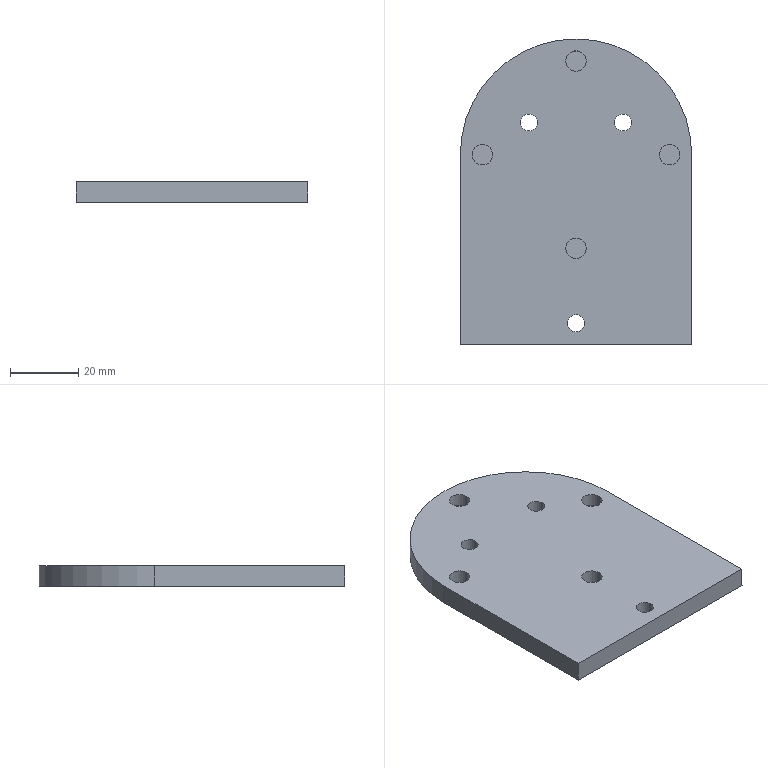Part | SolidWorks | features Cut 2, Extrusion 1 | 1 solid | 24 faces | box 68 x 89.927 x 6 mm | volume 32907 mm3 | cylinder 15 | plane 9 | commonest cylinder face diameters 6 x8 5 x6 68 x1
STEP:
#1=CARTESIAN_POINT('',(-43.159,19.21,6.));
#2=VERTEX_POINT('',#1);
#3=CARTESIAN_POINT('',(-48.159,19.21,6.));
#4=VERTEX_POINT('',#3);
#5=CARTESIAN_POINT('',(-45.659,19.21,6.));
#6=DIRECTION('',(0.,0.,-1.));
#7=DIRECTION('',(-1.,0.,0.));
#8=AXIS2_PLACEMENT_3D('',#5,#6,#7);
#9=CIRCLE('',#8,2.5);
#10=EDGE_CURVE('',#2,#4,#9,.T.);
#11=ORIENTED_EDGE('',*,*,#10,.F.);
#12=CARTESIAN_POINT('',(-43.159,19.21,0.));
#13=VERTEX_POINT('',#12);
#14=CARTESIAN_POINT('',(-43.159,19.21,6.));
#15=DIRECTION('',(0.,0.,-1.));
#16=VECTOR('',#15,1000.);
#17=LINE('',#14,#16);
#18=EDGE_CURVE('',#2,#13,#17,.T.);
#19=ORIENTED_EDGE('',*,*,#18,.T.);
#20=CARTESIAN_POINT('',(-48.159,19.21,0.));
#21=VERTEX_POINT('',#20);
#22=CARTESIAN_POINT('',(-45.659,19.21,0.));
#23=DIRECTION('',(0.,0.,-1.));
#24=DIRECTION('',(-1.,0.,0.));
#25=AXIS2_PLACEMENT_3D('',#22,#23,#24);
#26=CIRCLE('',#25,2.5);
#27=EDGE_CURVE('',#13,#21,#26,.T.);
#28=ORIENTED_EDGE('',*,*,#27,.T.);
#29=CARTESIAN_POINT('',(-48.159,19.21,6.));
#30=DIRECTION('',(0.,0.,-1.));
#31=VECTOR('',#30,1000.);
#32=LINE('',#29,#31);
#33=EDGE_CURVE('',#4,#21,#32,.T.);
#34=ORIENTED_EDGE('',*,*,#33,.F.);
#35=EDGE_LOOP('',(#11,#19,#28,#34));
#36=FACE_OUTER_BOUND('',#35,.T.);
#37=CARTESIAN_POINT('',(-45.659,19.21,6.));
#38=DIRECTION('',(0.,0.,-1.));
#39=DIRECTION('',(-1.,0.,0.));
#40=AXIS2_PLACEMENT_3D('',#37,#38,#39);
#41=CYLINDRICAL_SURFACE('',#40,2.5);
#42=ADVANCED_FACE('',(#36),#41,.F.);
#43=CARTESIAN_POINT('',(-15.478,19.21,6.));
#44=VERTEX_POINT('',#43);
#45=CARTESIAN_POINT('',(-20.478,19.21,6.));
#46=VERTEX_POINT('',#45);
#47=CARTESIAN_POINT('',(-17.978,19.21,6.));
#48=DIRECTION('',(0.,0.,-1.));
#49=DIRECTION('',(-1.,0.,0.));
#50=AXIS2_PLACEMENT_3D('',#47,#48,#49);
#51=CIRCLE('',#50,2.5);
#52=EDGE_CURVE('',#44,#46,#51,.T.);
#53=ORIENTED_EDGE('',*,*,#52,.F.);
#54=CARTESIAN_POINT('',(-15.478,19.21,0.));
#55=VERTEX_POINT('',#54);
#56=CARTESIAN_POINT('',(-15.478,19.21,6.));
#57=DIRECTION('',(0.,0.,-1.));
#58=VECTOR('',#57,1000.);
#59=LINE('',#56,#58);
#60=EDGE_CURVE('',#44,#55,#59,.T.);
#61=ORIENTED_EDGE('',*,*,#60,.T.);
#62=CARTESIAN_POINT('',(-20.478,19.21,0.));
#63=VERTEX_POINT('',#62);
#64=CARTESIAN_POINT('',(-17.978,19.21,0.));
#65=DIRECTION('',(0.,0.,-1.));
#66=DIRECTION('',(-1.,0.,0.));
#67=AXIS2_PLACEMENT_3D('',#64,#65,#66);
#68=CIRCLE('',#67,2.5);
#69=EDGE_CURVE('',#55,#63,#68,.T.);
#70=ORIENTED_EDGE('',*,*,#69,.T.);
#71=CARTESIAN_POINT('',(-20.478,19.21,6.));
#72=DIRECTION('',(0.,0.,-1.));
#73=VECTOR('',#72,1000.);
#74=LINE('',#71,#73);
#75=EDGE_CURVE('',#46,#63,#74,.T.);
#76=ORIENTED_EDGE('',*,*,#75,.F.);
#77=EDGE_LOOP('',(#53,#61,#70,#76));
#78=FACE_OUTER_BOUND('',#77,.T.);
#79=CARTESIAN_POINT('',(-17.978,19.21,6.));
#80=DIRECTION('',(0.,0.,-1.));
#81=DIRECTION('',(-1.,0.,0.));
#82=AXIS2_PLACEMENT_3D('',#79,#80,#81);
#83=CYLINDRICAL_SURFACE('',#82,2.5);
#84=ADVANCED_FACE('',(#78),#83,.F.);
#85=CARTESIAN_POINT('',(-29.318,-39.754,6.));
#86=VERTEX_POINT('',#85);
#87=CARTESIAN_POINT('',(-34.318,-39.754,6.));
#88=VERTEX_POINT('',#87);
#89=CARTESIAN_POINT('',(-31.818,-39.754,6.));
#90=DIRECTION('',(0.,0.,-1.));
#91=DIRECTION('',(-1.,0.,0.));
#92=AXIS2_PLACEMENT_3D('',#89,#90,#91);
#93=CIRCLE('',#92,2.5);
#94=EDGE_CURVE('',#86,#88,#93,.T.);
#95=ORIENTED_EDGE('',*,*,#94,.F.);
#96=CARTESIAN_POINT('',(-29.318,-39.754,0.));
#97=VERTEX_POINT('',#96);
#98=CARTESIAN_POINT('',(-29.318,-39.754,6.));
#99=DIRECTION('',(0.,0.,-1.));
#100=VECTOR('',#99,1000.);
#101=LINE('',#98,#100);
#102=EDGE_CURVE('',#86,#97,#101,.T.);
#103=ORIENTED_EDGE('',*,*,#102,.T.);
#104=CARTESIAN_POINT('',(-34.318,-39.754,0.));
#105=VERTEX_POINT('',#104);
#106=CARTESIAN_POINT('',(-31.818,-39.754,0.));
#107=DIRECTION('',(0.,0.,-1.));
#108=DIRECTION('',(-1.,0.,0.));
#109=AXIS2_PLACEMENT_3D('',#106,#107,#108);
#110=CIRCLE('',#109,2.5);
#111=EDGE_CURVE('',#97,#105,#110,.T.);
#112=ORIENTED_EDGE('',*,*,#111,.T.);
#113=CARTESIAN_POINT('',(-34.318,-39.754,6.));
#114=DIRECTION('',(0.,0.,-1.));
#115=VECTOR('',#114,1000.);
#116=LINE('',#113,#115);
#117=EDGE_CURVE('',#88,#105,#116,.T.);
#118=ORIENTED_EDGE('',*,*,#117,.F.);
#119=EDGE_LOOP('',(#95,#103,#112,#118));
#120=FACE_OUTER_BOUND('',#119,.T.);
#121=CARTESIAN_POINT('',(-31.818,-39.754,6.));
#122=DIRECTION('',(0.,0.,-1.));
#123=DIRECTION('',(-1.,0.,0.));
#124=AXIS2_PLACEMENT_3D('',#121,#122,#123);
#125=CYLINDRICAL_SURFACE('',#124,2.5);
#126=ADVANCED_FACE('',(#120),#125,.F.);
#127=CARTESIAN_POINT('',(-34.818,37.244,2.));
#128=VERTEX_POINT('',#127);
#129=CARTESIAN_POINT('',(-28.818,37.244,2.));
#130=VERTEX_POINT('',#129);
#131=CARTESIAN_POINT('',(-31.818,37.244,2.));
#132=DIRECTION('',(0.,0.,1.));
#133=DIRECTION('',(1.,0.,0.));
#134=AXIS2_PLACEMENT_3D('',#131,#132,#133);
#135=CIRCLE('',#134,3.);
#136=EDGE_CURVE('',#128,#130,#135,.T.);
#137=ORIENTED_EDGE('',*,*,#136,.F.);
#138=CARTESIAN_POINT('',(-34.818,37.244,6.));
#139=VERTEX_POINT('',#138);
#140=CARTESIAN_POINT('',(-34.818,37.244,2.));
#141=DIRECTION('',(0.,0.,1.));
#142=VECTOR('',#141,1000.);
#143=LINE('',#140,#142);
#144=EDGE_CURVE('',#128,#139,#143,.T.);
#145=ORIENTED_EDGE('',*,*,#144,.T.);
#146=CARTESIAN_POINT('',(-28.818,37.244,6.));
#147=VERTEX_POINT('',#146);
#148=CARTESIAN_POINT('',(-31.818,37.244,6.));
#149=DIRECTION('',(0.,0.,1.));
#150=DIRECTION('',(1.,0.,0.));
#151=AXIS2_PLACEMENT_3D('',#148,#149,#150);
#152=CIRCLE('',#151,3.);
#153=EDGE_CURVE('',#139,#147,#152,.T.);
#154=ORIENTED_EDGE('',*,*,#153,.T.);
#155=CARTESIAN_POINT('',(-28.818,37.244,2.));
#156=DIRECTION('',(0.,0.,1.));
#157=VECTOR('',#156,1000.);
#158=LINE('',#155,#157);
#159=EDGE_CURVE('',#130,#147,#158,.T.);
#160=ORIENTED_EDGE('',*,*,#159,.F.);
#161=EDGE_LOOP('',(#137,#145,#154,#160));
#162=FACE_OUTER_BOUND('',#161,.T.);
#163=CARTESIAN_POINT('',(-31.818,37.244,2.));
#164=DIRECTION('',(0.,0.,1.));
#165=DIRECTION('',(1.,0.,0.));
#166=AXIS2_PLACEMENT_3D('',#163,#164,#165);
#167=CYLINDRICAL_SURFACE('',#166,3.);
#168=ADVANCED_FACE('',(#162),#167,.F.);
#169=CARTESIAN_POINT('',(-7.318,9.744,2.));
#170=VERTEX_POINT('',#169);
#171=CARTESIAN_POINT('',(-1.318,9.744,2.));
#172=VERTEX_POINT('',#171);
#173=CARTESIAN_POINT('',(-4.318,9.744,2.));
#174=DIRECTION('',(0.,0.,1.));
#175=DIRECTION('',(1.,0.,0.));
#176=AXIS2_PLACEMENT_3D('',#173,#174,#175);
#177=CIRCLE('',#176,3.);
#178=EDGE_CURVE('',#170,#172,#177,.T.);
#179=ORIENTED_EDGE('',*,*,#178,.F.);
#180=CARTESIAN_POINT('',(-7.318,9.744,6.));
#181=VERTEX_POINT('',#180);
#182=CARTESIAN_POINT('',(-7.318,9.744,2.));
#183=DIRECTION('',(0.,0.,1.));
#184=VECTOR('',#183,1000.);
#185=LINE('',#182,#184);
#186=EDGE_CURVE('',#170,#181,#185,.T.);
#187=ORIENTED_EDGE('',*,*,#186,.T.);
#188=CARTESIAN_POINT('',(-1.318,9.744,6.));
#189=VERTEX_POINT('',#188);
#190=CARTESIAN_POINT('',(-4.318,9.744,6.));
#191=DIRECTION('',(0.,0.,1.));
#192=DIRECTION('',(1.,0.,0.));
#193=AXIS2_PLACEMENT_3D('',#190,#191,#192);
#194=CIRCLE('',#193,3.);
#195=EDGE_CURVE('',#181,#189,#194,.T.);
#196=ORIENTED_EDGE('',*,*,#195,.T.);
#197=CARTESIAN_POINT('',(-1.318,9.744,2.));
#198=DIRECTION('',(0.,0.,1.));
#199=VECTOR('',#198,1000.);
#200=LINE('',#197,#199);
#201=EDGE_CURVE('',#172,#189,#200,.T.);
#202=ORIENTED_EDGE('',*,*,#201,.F.);
#203=EDGE_LOOP('',(#179,#187,#196,#202));
#204=FACE_OUTER_BOUND('',#203,.T.);
#205=CARTESIAN_POINT('',(-4.318,9.744,2.));
#206=DIRECTION('',(0.,0.,1.));
#207=DIRECTION('',(1.,0.,0.));
#208=AXIS2_PLACEMENT_3D('',#205,#206,#207);
#209=CYLINDRICAL_SURFACE('',#208,3.);
#210=ADVANCED_FACE('',(#204),#209,.F.);
#211=CARTESIAN_POINT('',(-34.818,-17.756,2.));
#212=VERTEX_POINT('',#211);
#213=CARTESIAN_POINT('',(-28.818,-17.756,2.));
#214=VERTEX_POINT('',#213);
#215=CARTESIAN_POINT('',(-31.818,-17.756,2.));
#216=DIRECTION('',(0.,0.,1.));
#217=DIRECTION('',(1.,0.,0.));
#218=AXIS2_PLACEMENT_3D('',#215,#216,#217);
#219=CIRCLE('',#218,3.);
#220=EDGE_CURVE('',#212,#214,#219,.T.);
#221=ORIENTED_EDGE('',*,*,#220,.F.);
#222=CARTESIAN_POINT('',(-34.818,-17.756,6.));
#223=VERTEX_POINT('',#222);
#224=CARTESIAN_POINT('',(-34.818,-17.756,2.));
#225=DIRECTION('',(0.,0.,1.));
#226=VECTOR('',#225,1000.);
#227=LINE('',#224,#226);
#228=EDGE_CURVE('',#212,#223,#227,.T.);
#229=ORIENTED_EDGE('',*,*,#228,.T.);
#230=CARTESIAN_POINT('',(-28.818,-17.756,6.));
#231=VERTEX_POINT('',#230);
#232=CARTESIAN_POINT('',(-31.818,-17.756,6.));
#233=DIRECTION('',(0.,0.,1.));
#234=DIRECTION('',(1.,0.,0.));
#235=AXIS2_PLACEMENT_3D('',#232,#233,#234);
#236=CIRCLE('',#235,3.);
#237=EDGE_CURVE('',#223,#231,#236,.T.);
#238=ORIENTED_EDGE('',*,*,#237,.T.);
#239=CARTESIAN_POINT('',(-28.818,-17.756,2.));
#240=DIRECTION('',(0.,0.,1.));
#241=VECTOR('',#240,1000.);
#242=LINE('',#239,#241);
#243=EDGE_CURVE('',#214,#231,#242,.T.);
#244=ORIENTED_EDGE('',*,*,#243,.F.);
#245=EDGE_LOOP('',(#221,#229,#238,#244));
#246=FACE_OUTER_BOUND('',#245,.T.);
#247=CARTESIAN_POINT('',(-31.818,-17.756,2.));
#248=DIRECTION('',(0.,0.,1.));
#249=DIRECTION('',(1.,0.,0.));
#250=AXIS2_PLACEMENT_3D('',#247,#248,#249);
#251=CYLINDRICAL_SURFACE('',#250,3.);
#252=ADVANCED_FACE('',(#246),#251,.F.);
#253=CARTESIAN_POINT('',(-62.318,9.744,2.));
#254=VERTEX_POINT('',#253);
#255=CARTESIAN_POINT('',(-56.318,9.744,2.));
#256=VERTEX_POINT('',#255);
#257=CARTESIAN_POINT('',(-59.318,9.744,2.));
#258=DIRECTION('',(0.,0.,1.));
#259=DIRECTION('',(1.,0.,0.));
#260=AXIS2_PLACEMENT_3D('',#257,#258,#259);
#261=CIRCLE('',#260,3.);
#262=EDGE_CURVE('',#254,#256,#261,.T.);
#263=ORIENTED_EDGE('',*,*,#262,.F.);
#264=CARTESIAN_POINT('',(-62.318,9.744,6.));
#265=VERTEX_POINT('',#264);
#266=CARTESIAN_POINT('',(-62.318,9.744,2.));
#267=DIRECTION('',(0.,0.,1.));
#268=VECTOR('',#267,1000.);
#269=LINE('',#266,#268);
#270=EDGE_CURVE('',#254,#265,#269,.T.);
#271=ORIENTED_EDGE('',*,*,#270,.T.);
#272=CARTESIAN_POINT('',(-56.318,9.744,6.));
#273=VERTEX_POINT('',#272);
#274=CARTESIAN_POINT('',(-59.318,9.744,6.));
#275=DIRECTION('',(0.,0.,1.));
#276=DIRECTION('',(1.,0.,0.));
#277=AXIS2_PLACEMENT_3D('',#274,#275,#276);
#278=CIRCLE('',#277,3.);
#279=EDGE_CURVE('',#265,#273,#278,.T.);
#280=ORIENTED_EDGE('',*,*,#279,.T.);
#281=CARTESIAN_POINT('',(-56.318,9.744,2.));
#282=DIRECTION('',(0.,0.,1.));
#283=VECTOR('',#282,1000.);
#284=LINE('',#281,#283);
#285=EDGE_CURVE('',#256,#273,#284,.T.);
#286=ORIENTED_EDGE('',*,*,#285,.F.);
#287=EDGE_LOOP('',(#263,#271,#280,#286));
#288=FACE_OUTER_BOUND('',#287,.T.);
#289=CARTESIAN_POINT('',(-59.318,9.744,2.));
#290=DIRECTION('',(0.,0.,1.));
#291=DIRECTION('',(1.,0.,0.));
#292=AXIS2_PLACEMENT_3D('',#289,#290,#291);
#293=CYLINDRICAL_SURFACE('',#292,3.);
#294=ADVANCED_FACE('',(#288),#293,.F.);
#295=CARTESIAN_POINT('',(2.182,9.744,0.));
#296=VERTEX_POINT('',#295);
#297=CARTESIAN_POINT('',(-65.818,9.744,0.));
#298=VERTEX_POINT('',#297);
#299=CARTESIAN_POINT('',(-31.818,9.744,0.));
#300=DIRECTION('',(0.,0.,1.));
#301=DIRECTION('',(1.,0.,0.));
#302=AXIS2_PLACEMENT_3D('',#299,#300,#301);
#303=CIRCLE('',#302,34.);
#304=EDGE_CURVE('',#296,#298,#303,.T.);
#305=ORIENTED_EDGE('',*,*,#304,.T.);
#306=CARTESIAN_POINT('',(-65.818,9.744,6.));
#307=VERTEX_POINT('',#306);
#308=CARTESIAN_POINT('',(-65.818,9.744,6.));
#309=DIRECTION('',(0.,0.,-1.));
#310=VECTOR('',#309,1000.);
#311=LINE('',#308,#310);
#312=EDGE_CURVE('',#307,#298,#311,.T.);
#313=ORIENTED_EDGE('',*,*,#312,.F.);
#314=CARTESIAN_POINT('',(2.182,9.744,6.));
#315=VERTEX_POINT('',#314);
#316=CARTESIAN_POINT('',(-31.818,9.744,6.));
#317=DIRECTION('',(0.,0.,1.));
#318=DIRECTION('',(1.,0.,0.));
#319=AXIS2_PLACEMENT_3D('',#316,#317,#318);
#320=CIRCLE('',#319,34.);
#321=EDGE_CURVE('',#315,#307,#320,.T.);
#322=ORIENTED_EDGE('',*,*,#321,.F.);
#323=CARTESIAN_POINT('',(2.182,9.744,6.));
#324=DIRECTION('',(0.,0.,-1.));
#325=VECTOR('',#324,1000.);
#326=LINE('',#323,#325);
#327=EDGE_CURVE('',#315,#296,#326,.T.);
#328=ORIENTED_EDGE('',*,*,#327,.T.);
#329=EDGE_LOOP('',(#305,#313,#322,#328));
#330=FACE_OUTER_BOUND('',#329,.T.);
#331=CARTESIAN_POINT('',(-31.818,9.744,6.));
#332=DIRECTION('',(0.,0.,-1.));
#333=DIRECTION('',(-1.,0.,0.));
#334=AXIS2_PLACEMENT_3D('',#331,#332,#333);
#335=CYLINDRICAL_SURFACE('',#334,34.);
#336=ADVANCED_FACE('',(#330),#335,.T.);
#337=CARTESIAN_POINT('',(-65.818,-46.183,0.));
#338=VERTEX_POINT('',#337);
#339=CARTESIAN_POINT('',(-65.818,-46.183,0.));
#340=DIRECTION('',(0.,-1.,0.));
#341=VECTOR('',#340,1000.);
#342=LINE('',#339,#341);
#343=EDGE_CURVE('',#298,#338,#342,.T.);
#344=ORIENTED_EDGE('',*,*,#343,.T.);
#345=CARTESIAN_POINT('',(-65.818,-46.183,6.));
#346=VERTEX_POINT('',#345);
#347=CARTESIAN_POINT('',(-65.818,-46.183,6.));
#348=DIRECTION('',(0.,0.,-1.));
#349=VECTOR('',#348,1000.);
#350=LINE('',#347,#349);
#351=EDGE_CURVE('',#346,#338,#350,.T.);
#352=ORIENTED_EDGE('',*,*,#351,.F.);
#353=CARTESIAN_POINT('',(-65.818,-46.183,6.));
#354=DIRECTION('',(0.,-1.,0.));
#355=VECTOR('',#354,1000.);
#356=LINE('',#353,#355);
#357=EDGE_CURVE('',#307,#346,#356,.T.);
#358=ORIENTED_EDGE('',*,*,#357,.F.);
#359=ORIENTED_EDGE('',*,*,#312,.T.);
#360=EDGE_LOOP('',(#344,#352,#358,#359));
#361=FACE_OUTER_BOUND('',#360,.T.);
#362=CARTESIAN_POINT('',(-65.818,-46.183,6.));
#363=DIRECTION('',(1.,0.,0.));
#364=DIRECTION('',(0.,0.,-1.));
#365=AXIS2_PLACEMENT_3D('',#362,#363,#364);
#366=PLANE('',#365);
#367=ADVANCED_FACE('',(#361),#366,.F.);
#368=CARTESIAN_POINT('',(2.182,-46.183,0.));
#369=VERTEX_POINT('',#368);
#370=CARTESIAN_POINT('',(2.182,-46.183,0.));
#371=DIRECTION('',(1.,0.,0.));
#372=VECTOR('',#371,1000.);
#373=LINE('',#370,#372);
#374=EDGE_CURVE('',#338,#369,#373,.T.);
#375=ORIENTED_EDGE('',*,*,#374,.T.);
#376=CARTESIAN_POINT('',(2.182,-46.183,6.));
#377=VERTEX_POINT('',#376);
#378=CARTESIAN_POINT('',(2.182,-46.183,6.));
#379=DIRECTION('',(0.,0.,-1.));
#380=VECTOR('',#379,1000.);
#381=LINE('',#378,#380);
#382=EDGE_CURVE('',#377,#369,#381,.T.);
#383=ORIENTED_EDGE('',*,*,#382,.F.);
#384=CARTESIAN_POINT('',(2.182,-46.183,6.));
#385=DIRECTION('',(1.,0.,0.));
#386=VECTOR('',#385,1000.);
#387=LINE('',#384,#386);
#388=EDGE_CURVE('',#346,#377,#387,.T.);
#389=ORIENTED_EDGE('',*,*,#388,.F.);
#390=ORIENTED_EDGE('',*,*,#351,.T.);
#391=EDGE_LOOP('',(#375,#383,#389,#390));
#392=FACE_OUTER_BOUND('',#391,.T.);
#393=CARTESIAN_POINT('',(2.182,-46.183,6.));
#394=DIRECTION('',(0.,1.,0.));
#395=DIRECTION('',(-1.,0.,0.));
#396=AXIS2_PLACEMENT_3D('',#393,#394,#395);
#397=PLANE('',#396);
#398=ADVANCED_FACE('',(#392),#397,.F.);
#399=CARTESIAN_POINT('',(2.182,9.744,0.));
#400=DIRECTION('',(0.,1.,0.));
#401=VECTOR('',#400,1000.);
#402=LINE('',#399,#401);
#403=EDGE_CURVE('',#369,#296,#402,.T.);
#404=ORIENTED_EDGE('',*,*,#403,.T.);
#405=ORIENTED_EDGE('',*,*,#327,.F.);
#406=CARTESIAN_POINT('',(2.182,9.744,6.));
#407=DIRECTION('',(0.,1.,0.));
#408=VECTOR('',#407,1000.);
#409=LINE('',#406,#408);
#410=EDGE_CURVE('',#377,#315,#409,.T.);
#411=ORIENTED_EDGE('',*,*,#410,.F.);
#412=ORIENTED_EDGE('',*,*,#382,.T.);
#413=EDGE_LOOP('',(#404,#405,#411,#412));
#414=FACE_OUTER_BOUND('',#413,.T.);
#415=CARTESIAN_POINT('',(2.182,9.744,6.));
#416=DIRECTION('',(-1.,0.,0.));
#417=DIRECTION('',(0.,-1.,0.));
#418=AXIS2_PLACEMENT_3D('',#415,#416,#417);
#419=PLANE('',#418);
#420=ADVANCED_FACE('',(#414),#419,.F.);
#421=CARTESIAN_POINT('',(-45.659,19.21,6.));
#422=DIRECTION('',(0.,0.,-1.));
#423=DIRECTION('',(-1.,0.,0.));
#424=AXIS2_PLACEMENT_3D('',#421,#422,#423);
#425=CIRCLE('',#424,2.5);
#426=EDGE_CURVE('',#4,#2,#425,.T.);
#427=ORIENTED_EDGE('',*,*,#426,.T.);
#428=ORIENTED_EDGE('',*,*,#10,.T.);
#429=EDGE_LOOP('',(#427,#428));
#430=FACE_BOUND('',#429,.T.);
#431=CARTESIAN_POINT('',(-17.978,19.21,6.));
#432=DIRECTION('',(0.,0.,-1.));
#433=DIRECTION('',(-1.,0.,0.));
#434=AXIS2_PLACEMENT_3D('',#431,#432,#433);
#435=CIRCLE('',#434,2.5);
#436=EDGE_CURVE('',#46,#44,#435,.T.);
#437=ORIENTED_EDGE('',*,*,#436,.T.);
#438=ORIENTED_EDGE('',*,*,#52,.T.);
#439=EDGE_LOOP('',(#437,#438));
#440=FACE_BOUND('',#439,.T.);
#441=CARTESIAN_POINT('',(-31.818,-39.754,6.));
#442=DIRECTION('',(0.,0.,-1.));
#443=DIRECTION('',(-1.,0.,0.));
#444=AXIS2_PLACEMENT_3D('',#441,#442,#443);
#445=CIRCLE('',#444,2.5);
#446=EDGE_CURVE('',#88,#86,#445,.T.);
#447=ORIENTED_EDGE('',*,*,#446,.T.);
#448=ORIENTED_EDGE('',*,*,#94,.T.);
#449=EDGE_LOOP('',(#447,#448));
#450=FACE_BOUND('',#449,.T.);
#451=CARTESIAN_POINT('',(-31.818,37.244,6.));
#452=DIRECTION('',(0.,0.,1.));
#453=DIRECTION('',(1.,0.,0.));
#454=AXIS2_PLACEMENT_3D('',#451,#452,#453);
#455=CIRCLE('',#454,3.);
#456=EDGE_CURVE('',#147,#139,#455,.T.);
#457=ORIENTED_EDGE('',*,*,#456,.F.);
#458=ORIENTED_EDGE('',*,*,#153,.F.);
#459=EDGE_LOOP('',(#457,#458));
#460=FACE_BOUND('',#459,.T.);
#461=CARTESIAN_POINT('',(-4.318,9.744,6.));
#462=DIRECTION('',(0.,0.,1.));
#463=DIRECTION('',(1.,0.,0.));
#464=AXIS2_PLACEMENT_3D('',#461,#462,#463);
#465=CIRCLE('',#464,3.);
#466=EDGE_CURVE('',#189,#181,#465,.T.);
#467=ORIENTED_EDGE('',*,*,#466,.F.);
#468=ORIENTED_EDGE('',*,*,#195,.F.);
#469=EDGE_LOOP('',(#467,#468));
#470=FACE_BOUND('',#469,.T.);
#471=CARTESIAN_POINT('',(-31.818,-17.756,6.));
#472=DIRECTION('',(0.,0.,1.));
#473=DIRECTION('',(1.,0.,0.));
#474=AXIS2_PLACEMENT_3D('',#471,#472,#473);
#475=CIRCLE('',#474,3.);
#476=EDGE_CURVE('',#231,#223,#475,.T.);
#477=ORIENTED_EDGE('',*,*,#476,.F.);
#478=ORIENTED_EDGE('',*,*,#237,.F.);
#479=EDGE_LOOP('',(#477,#478));
#480=FACE_BOUND('',#479,.T.);
#481=CARTESIAN_POINT('',(-59.318,9.744,6.));
#482=DIRECTION('',(0.,0.,1.));
#483=DIRECTION('',(1.,0.,0.));
#484=AXIS2_PLACEMENT_3D('',#481,#482,#483);
#485=CIRCLE('',#484,3.);
#486=EDGE_CURVE('',#273,#265,#485,.T.);
#487=ORIENTED_EDGE('',*,*,#486,.F.);
#488=ORIENTED_EDGE('',*,*,#279,.F.);
#489=EDGE_LOOP('',(#487,#488));
#490=FACE_BOUND('',#489,.T.);
#491=ORIENTED_EDGE('',*,*,#321,.T.);
#492=ORIENTED_EDGE('',*,*,#357,.T.);
#493=ORIENTED_EDGE('',*,*,#388,.T.);
#494=ORIENTED_EDGE('',*,*,#410,.T.);
#495=EDGE_LOOP('',(#491,#492,#493,#494));
#496=FACE_OUTER_BOUND('',#495,.T.);
#497=CARTESIAN_POINT('',(-31.818,9.744,6.));
#498=DIRECTION('',(0.,0.,1.));
#499=DIRECTION('',(1.,0.,0.));
#500=AXIS2_PLACEMENT_3D('',#497,#498,#499);
#501=PLANE('',#500);
#502=ADVANCED_FACE('',(#430,#440,#450,#460,#470,#480,#490,#496),#501,.T.);
#503=CARTESIAN_POINT('',(-45.659,19.21,0.));
#504=DIRECTION('',(0.,0.,-1.));
#505=DIRECTION('',(-1.,0.,0.));
#506=AXIS2_PLACEMENT_3D('',#503,#504,#505);
#507=CIRCLE('',#506,2.5);
#508=EDGE_CURVE('',#21,#13,#507,.T.);
#509=ORIENTED_EDGE('',*,*,#508,.F.);
#510=ORIENTED_EDGE('',*,*,#27,.F.);
#511=EDGE_LOOP('',(#509,#510));
#512=FACE_BOUND('',#511,.T.);
#513=CARTESIAN_POINT('',(-17.978,19.21,0.));
#514=DIRECTION('',(0.,0.,-1.));
#515=DIRECTION('',(-1.,0.,0.));
#516=AXIS2_PLACEMENT_3D('',#513,#514,#515);
#517=CIRCLE('',#516,2.5);
#518=EDGE_CURVE('',#63,#55,#517,.T.);
#519=ORIENTED_EDGE('',*,*,#518,.F.);
#520=ORIENTED_EDGE('',*,*,#69,.F.);
#521=EDGE_LOOP('',(#519,#520));
#522=FACE_BOUND('',#521,.T.);
#523=CARTESIAN_POINT('',(-31.818,-39.754,0.));
#524=DIRECTION('',(0.,0.,-1.));
#525=DIRECTION('',(-1.,0.,0.));
#526=AXIS2_PLACEMENT_3D('',#523,#524,#525);
#527=CIRCLE('',#526,2.5);
#528=EDGE_CURVE('',#105,#97,#527,.T.);
#529=ORIENTED_EDGE('',*,*,#528,.F.);
#530=ORIENTED_EDGE('',*,*,#111,.F.);
#531=EDGE_LOOP('',(#529,#530));
#532=FACE_BOUND('',#531,.T.);
#533=ORIENTED_EDGE('',*,*,#304,.F.);
#534=ORIENTED_EDGE('',*,*,#403,.F.);
#535=ORIENTED_EDGE('',*,*,#374,.F.);
#536=ORIENTED_EDGE('',*,*,#343,.F.);
#537=EDGE_LOOP('',(#533,#534,#535,#536));
#538=FACE_OUTER_BOUND('',#537,.T.);
#539=CARTESIAN_POINT('',(-31.818,9.744,0.));
#540=DIRECTION('',(0.,0.,1.));
#541=DIRECTION('',(1.,0.,0.));
#542=AXIS2_PLACEMENT_3D('',#539,#540,#541);
#543=PLANE('',#542);
#544=ADVANCED_FACE('',(#512,#522,#532,#538),#543,.F.);
#545=ORIENTED_EDGE('',*,*,#270,.F.);
#546=CARTESIAN_POINT('',(-59.318,9.744,2.));
#547=DIRECTION('',(0.,0.,1.));
#548=DIRECTION('',(1.,0.,0.));
#549=AXIS2_PLACEMENT_3D('',#546,#547,#548);
#550=CIRCLE('',#549,3.);
#551=EDGE_CURVE('',#256,#254,#550,.T.);
#552=ORIENTED_EDGE('',*,*,#551,.F.);
#553=ORIENTED_EDGE('',*,*,#285,.T.);
#554=ORIENTED_EDGE('',*,*,#486,.T.);
#555=EDGE_LOOP('',(#545,#552,#553,#554));
#556=FACE_OUTER_BOUND('',#555,.T.);
#557=CARTESIAN_POINT('',(-59.318,9.744,2.));
#558=DIRECTION('',(0.,0.,1.));
#559=DIRECTION('',(1.,0.,0.));
#560=AXIS2_PLACEMENT_3D('',#557,#558,#559);
#561=CYLINDRICAL_SURFACE('',#560,3.);
#562=ADVANCED_FACE('',(#556),#561,.F.);
#563=ORIENTED_EDGE('',*,*,#551,.T.);
#564=ORIENTED_EDGE('',*,*,#262,.T.);
#565=EDGE_LOOP('',(#563,#564));
#566=FACE_OUTER_BOUND('',#565,.T.);
#567=CARTESIAN_POINT('',(0.,0.,2.));
#568=DIRECTION('',(0.,0.,1.));
#569=DIRECTION('',(1.,0.,0.));
#570=AXIS2_PLACEMENT_3D('',#567,#568,#569);
#571=PLANE('',#570);
#572=ADVANCED_FACE('',(#566),#571,.T.);
#573=ORIENTED_EDGE('',*,*,#228,.F.);
#574=CARTESIAN_POINT('',(-31.818,-17.756,2.));
#575=DIRECTION('',(0.,0.,1.));
#576=DIRECTION('',(1.,0.,0.));
#577=AXIS2_PLACEMENT_3D('',#574,#575,#576);
#578=CIRCLE('',#577,3.);
#579=EDGE_CURVE('',#214,#212,#578,.T.);
#580=ORIENTED_EDGE('',*,*,#579,.F.);
#581=ORIENTED_EDGE('',*,*,#243,.T.);
#582=ORIENTED_EDGE('',*,*,#476,.T.);
#583=EDGE_LOOP('',(#573,#580,#581,#582));
#584=FACE_OUTER_BOUND('',#583,.T.);
#585=CARTESIAN_POINT('',(-31.818,-17.756,2.));
#586=DIRECTION('',(0.,0.,1.));
#587=DIRECTION('',(1.,0.,0.));
#588=AXIS2_PLACEMENT_3D('',#585,#586,#587);
#589=CYLINDRICAL_SURFACE('',#588,3.);
#590=ADVANCED_FACE('',(#584),#589,.F.);
#591=ORIENTED_EDGE('',*,*,#579,.T.);
#592=ORIENTED_EDGE('',*,*,#220,.T.);
#593=EDGE_LOOP('',(#591,#592));
#594=FACE_OUTER_BOUND('',#593,.T.);
#595=CARTESIAN_POINT('',(0.,0.,2.));
#596=DIRECTION('',(0.,0.,1.));
#597=DIRECTION('',(1.,0.,0.));
#598=AXIS2_PLACEMENT_3D('',#595,#596,#597);
#599=PLANE('',#598);
#600=ADVANCED_FACE('',(#594),#599,.T.);
#601=ORIENTED_EDGE('',*,*,#186,.F.);
#602=CARTESIAN_POINT('',(-4.318,9.744,2.));
#603=DIRECTION('',(0.,0.,1.));
#604=DIRECTION('',(1.,0.,0.));
#605=AXIS2_PLACEMENT_3D('',#602,#603,#604);
#606=CIRCLE('',#605,3.);
#607=EDGE_CURVE('',#172,#170,#606,.T.);
#608=ORIENTED_EDGE('',*,*,#607,.F.);
#609=ORIENTED_EDGE('',*,*,#201,.T.);
#610=ORIENTED_EDGE('',*,*,#466,.T.);
#611=EDGE_LOOP('',(#601,#608,#609,#610));
#612=FACE_OUTER_BOUND('',#611,.T.);
#613=CARTESIAN_POINT('',(-4.318,9.744,2.));
#614=DIRECTION('',(0.,0.,1.));
#615=DIRECTION('',(1.,0.,0.));
#616=AXIS2_PLACEMENT_3D('',#613,#614,#615);
#617=CYLINDRICAL_SURFACE('',#616,3.);
#618=ADVANCED_FACE('',(#612),#617,.F.);
#619=ORIENTED_EDGE('',*,*,#607,.T.);
#620=ORIENTED_EDGE('',*,*,#178,.T.);
#621=EDGE_LOOP('',(#619,#620));
#622=FACE_OUTER_BOUND('',#621,.T.);
#623=CARTESIAN_POINT('',(0.,0.,2.));
#624=DIRECTION('',(0.,0.,1.));
#625=DIRECTION('',(1.,0.,0.));
#626=AXIS2_PLACEMENT_3D('',#623,#624,#625);
#627=PLANE('',#626);
#628=ADVANCED_FACE('',(#622),#627,.T.);
#629=ORIENTED_EDGE('',*,*,#144,.F.);
#630=CARTESIAN_POINT('',(-31.818,37.244,2.));
#631=DIRECTION('',(0.,0.,1.));
#632=DIRECTION('',(1.,0.,0.));
#633=AXIS2_PLACEMENT_3D('',#630,#631,#632);
#634=CIRCLE('',#633,3.);
#635=EDGE_CURVE('',#130,#128,#634,.T.);
#636=ORIENTED_EDGE('',*,*,#635,.F.);
#637=ORIENTED_EDGE('',*,*,#159,.T.);
#638=ORIENTED_EDGE('',*,*,#456,.T.);
#639=EDGE_LOOP('',(#629,#636,#637,#638));
#640=FACE_OUTER_BOUND('',#639,.T.);
#641=CARTESIAN_POINT('',(-31.818,37.244,2.));
#642=DIRECTION('',(0.,0.,1.));
#643=DIRECTION('',(1.,0.,0.));
#644=AXIS2_PLACEMENT_3D('',#641,#642,#643);
#645=CYLINDRICAL_SURFACE('',#644,3.);
#646=ADVANCED_FACE('',(#640),#645,.F.);
#647=ORIENTED_EDGE('',*,*,#635,.T.);
#648=ORIENTED_EDGE('',*,*,#136,.T.);
#649=EDGE_LOOP('',(#647,#648));
#650=FACE_OUTER_BOUND('',#649,.T.);
#651=CARTESIAN_POINT('',(0.,0.,2.));
#652=DIRECTION('',(0.,0.,1.));
#653=DIRECTION('',(1.,0.,0.));
#654=AXIS2_PLACEMENT_3D('',#651,#652,#653);
#655=PLANE('',#654);
#656=ADVANCED_FACE('',(#650),#655,.T.);
#657=ORIENTED_EDGE('',*,*,#102,.F.);
#658=ORIENTED_EDGE('',*,*,#446,.F.);
#659=ORIENTED_EDGE('',*,*,#117,.T.);
#660=ORIENTED_EDGE('',*,*,#528,.T.);
#661=EDGE_LOOP('',(#657,#658,#659,#660));
#662=FACE_OUTER_BOUND('',#661,.T.);
#663=CARTESIAN_POINT('',(-31.818,-39.754,6.));
#664=DIRECTION('',(0.,0.,-1.));
#665=DIRECTION('',(-1.,0.,0.));
#666=AXIS2_PLACEMENT_3D('',#663,#664,#665);
#667=CYLINDRICAL_SURFACE('',#666,2.5);
#668=ADVANCED_FACE('',(#662),#667,.F.);
#669=ORIENTED_EDGE('',*,*,#60,.F.);
#670=ORIENTED_EDGE('',*,*,#436,.F.);
#671=ORIENTED_EDGE('',*,*,#75,.T.);
#672=ORIENTED_EDGE('',*,*,#518,.T.);
#673=EDGE_LOOP('',(#669,#670,#671,#672));
#674=FACE_OUTER_BOUND('',#673,.T.);
#675=CARTESIAN_POINT('',(-17.978,19.21,6.));
#676=DIRECTION('',(0.,0.,-1.));
#677=DIRECTION('',(-1.,0.,0.));
#678=AXIS2_PLACEMENT_3D('',#675,#676,#677);
#679=CYLINDRICAL_SURFACE('',#678,2.5);
#680=ADVANCED_FACE('',(#674),#679,.F.);
#681=ORIENTED_EDGE('',*,*,#18,.F.);
#682=ORIENTED_EDGE('',*,*,#426,.F.);
#683=ORIENTED_EDGE('',*,*,#33,.T.);
#684=ORIENTED_EDGE('',*,*,#508,.T.);
#685=EDGE_LOOP('',(#681,#682,#683,#684));
#686=FACE_OUTER_BOUND('',#685,.T.);
#687=CARTESIAN_POINT('',(-45.659,19.21,6.));
#688=DIRECTION('',(0.,0.,-1.));
#689=DIRECTION('',(-1.,0.,0.));
#690=AXIS2_PLACEMENT_3D('',#687,#688,#689);
#691=CYLINDRICAL_SURFACE('',#690,2.5);
#692=ADVANCED_FACE('',(#686),#691,.F.);
#693=CLOSED_SHELL('',(#42,#84,#126,#168,#210,#252,#294,#336,#367,#398,#420,#502,#544,#562,#572,#590,#600,#618,#628,#646,#656,#668,#680,#692));
#694=MANIFOLD_SOLID_BREP('',#693);
#695=CARTESIAN_POINT('',(0.,0.,0.));
#696=DIRECTION('',(0.,0.,1.));
#697=DIRECTION('',(1.,0.,0.));
#698=AXIS2_PLACEMENT_3D('',#695,#696,#697);
#699=(LENGTH_UNIT()NAMED_UNIT(*)SI_UNIT(.MILLI.,.METRE.));
#700=UNCERTAINTY_MEASURE_WITH_UNIT(LENGTH_MEASURE(0.00001),#699,'','');
#701=(NAMED_UNIT(*)PLANE_ANGLE_UNIT()SI_UNIT($,.RADIAN.));
#702=(NAMED_UNIT(*)SI_UNIT($,.STERADIAN.)SOLID_ANGLE_UNIT());
#703=(GEOMETRIC_REPRESENTATION_CONTEXT(3)GLOBAL_UNCERTAINTY_ASSIGNED_CONTEXT((#700))GLOBAL_UNIT_ASSIGNED_CONTEXT((#699,#701,#702))REPRESENTATION_CONTEXT('',''));
#704=ADVANCED_BREP_SHAPE_REPRESENTATION('',(#694,#698),#703);